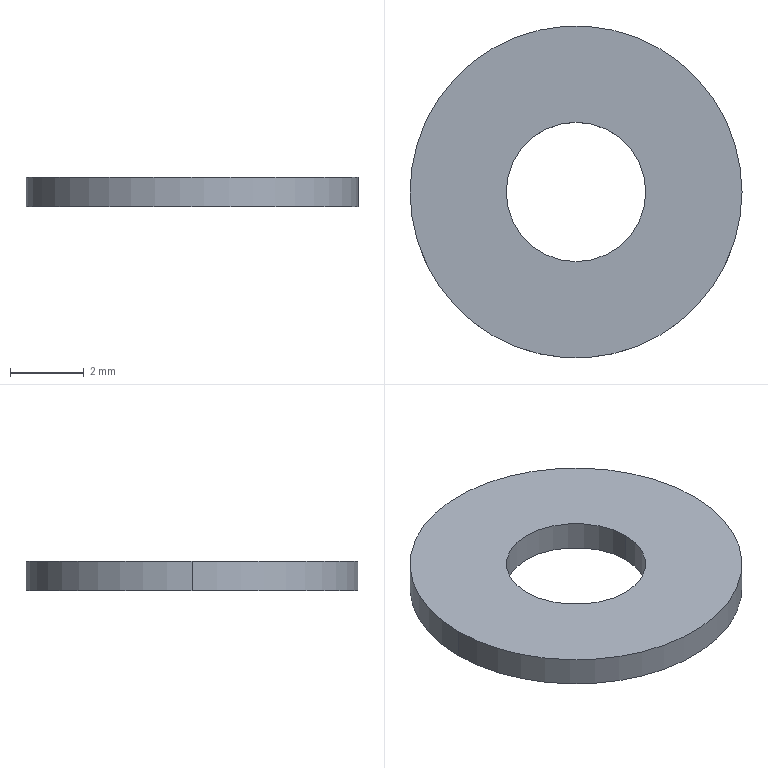Part | NX | features BREP 1 | 1 solid | 6 faces | box 9 x 9 x 0.8 mm | volume 41.916 mm3 | cylinder 4 | plane 2 | commonest cylinder face diameters 3.78 x2 9 x2
STEP:
#1=CARTESIAN_POINT('',(-264.811,-198.403,2105.2));
#2=VERTEX_POINT('',#1);
#3=CARTESIAN_POINT('',(-255.811,-198.403,2105.2));
#4=VERTEX_POINT('',#3);
#5=CARTESIAN_POINT('',(-260.311,-198.403,2105.2));
#6=DIRECTION('',(0.,0.,-1.));
#7=DIRECTION('',(1.,0.,0.));
#8=AXIS2_PLACEMENT_3D('',#5,#6,#7);
#9=CIRCLE('',#8,4.5);
#10=EDGE_CURVE('',#2,#4,#9,.T.);
#11=ORIENTED_EDGE('',*,*,#10,.F.);
#12=CARTESIAN_POINT('',(-264.811,-198.403,2106.));
#13=VERTEX_POINT('',#12);
#14=CARTESIAN_POINT('',(-264.811,-198.403,2106.));
#15=DIRECTION('',(0.,0.,1.));
#16=VECTOR('',#15,1000.);
#17=LINE('',#14,#16);
#18=EDGE_CURVE('',#2,#13,#17,.T.);
#19=ORIENTED_EDGE('',*,*,#18,.T.);
#20=CARTESIAN_POINT('',(-255.811,-198.403,2106.));
#21=VERTEX_POINT('',#20);
#22=CARTESIAN_POINT('',(-260.311,-198.403,2106.));
#23=DIRECTION('',(0.,0.,-1.));
#24=DIRECTION('',(1.,0.,0.));
#25=AXIS2_PLACEMENT_3D('',#22,#23,#24);
#26=CIRCLE('',#25,4.5);
#27=EDGE_CURVE('',#13,#21,#26,.T.);
#28=ORIENTED_EDGE('',*,*,#27,.T.);
#29=CARTESIAN_POINT('',(-255.811,-198.403,2106.));
#30=DIRECTION('',(0.,0.,1.));
#31=VECTOR('',#30,1000.);
#32=LINE('',#29,#31);
#33=EDGE_CURVE('',#4,#21,#32,.T.);
#34=ORIENTED_EDGE('',*,*,#33,.F.);
#35=EDGE_LOOP('',(#11,#19,#28,#34));
#36=FACE_BOUND('',#35,.T.);
#37=CARTESIAN_POINT('',(-260.311,-198.403,2106.));
#38=DIRECTION('',(0.,0.,1.));
#39=DIRECTION('',(-1.,0.,0.));
#40=AXIS2_PLACEMENT_3D('',#37,#38,#39);
#41=CYLINDRICAL_SURFACE('',#40,4.5);
#42=ADVANCED_FACE('',(#36),#41,.T.);
#43=CARTESIAN_POINT('',(-262.201,-198.403,2105.2));
#44=VERTEX_POINT('',#43);
#45=CARTESIAN_POINT('',(-258.421,-198.403,2105.2));
#46=VERTEX_POINT('',#45);
#47=CARTESIAN_POINT('',(-260.311,-198.403,2105.2));
#48=DIRECTION('',(0.,0.,1.));
#49=DIRECTION('',(1.,0.,0.));
#50=AXIS2_PLACEMENT_3D('',#47,#48,#49);
#51=CIRCLE('',#50,1.89);
#52=EDGE_CURVE('',#44,#46,#51,.T.);
#53=ORIENTED_EDGE('',*,*,#52,.F.);
#54=CARTESIAN_POINT('',(-262.201,-198.403,2106.));
#55=VERTEX_POINT('',#54);
#56=CARTESIAN_POINT('',(-262.201,-198.403,2106.));
#57=DIRECTION('',(0.,0.,1.));
#58=VECTOR('',#57,1000.);
#59=LINE('',#56,#58);
#60=EDGE_CURVE('',#44,#55,#59,.T.);
#61=ORIENTED_EDGE('',*,*,#60,.T.);
#62=CARTESIAN_POINT('',(-258.421,-198.403,2106.));
#63=VERTEX_POINT('',#62);
#64=CARTESIAN_POINT('',(-260.311,-198.403,2106.));
#65=DIRECTION('',(0.,0.,-1.));
#66=DIRECTION('',(1.,0.,0.));
#67=AXIS2_PLACEMENT_3D('',#64,#65,#66);
#68=CIRCLE('',#67,1.89);
#69=EDGE_CURVE('',#63,#55,#68,.T.);
#70=ORIENTED_EDGE('',*,*,#69,.F.);
#71=CARTESIAN_POINT('',(-258.421,-198.403,2106.));
#72=DIRECTION('',(0.,0.,1.));
#73=VECTOR('',#72,1000.);
#74=LINE('',#71,#73);
#75=EDGE_CURVE('',#46,#63,#74,.T.);
#76=ORIENTED_EDGE('',*,*,#75,.F.);
#77=EDGE_LOOP('',(#53,#61,#70,#76));
#78=FACE_BOUND('',#77,.T.);
#79=CARTESIAN_POINT('',(-260.311,-198.403,2106.));
#80=DIRECTION('',(0.,0.,1.));
#81=DIRECTION('',(-1.,0.,0.));
#82=AXIS2_PLACEMENT_3D('',#79,#80,#81);
#83=CYLINDRICAL_SURFACE('',#82,1.89);
#84=ADVANCED_FACE('',(#78),#83,.F.);
#85=CARTESIAN_POINT('',(-260.311,-198.403,2105.2));
#86=DIRECTION('',(0.,0.,-1.));
#87=DIRECTION('',(1.,0.,0.));
#88=AXIS2_PLACEMENT_3D('',#85,#86,#87);
#89=CIRCLE('',#88,4.5);
#90=EDGE_CURVE('',#4,#2,#89,.T.);
#91=ORIENTED_EDGE('',*,*,#90,.T.);
#92=ORIENTED_EDGE('',*,*,#10,.T.);
#93=EDGE_LOOP('',(#91,#92));
#94=FACE_BOUND('',#93,.T.);
#95=CARTESIAN_POINT('',(-260.311,-198.403,2105.2));
#96=DIRECTION('',(0.,0.,1.));
#97=DIRECTION('',(1.,0.,0.));
#98=AXIS2_PLACEMENT_3D('',#95,#96,#97);
#99=CIRCLE('',#98,1.89);
#100=EDGE_CURVE('',#46,#44,#99,.T.);
#101=ORIENTED_EDGE('',*,*,#100,.T.);
#102=ORIENTED_EDGE('',*,*,#52,.T.);
#103=EDGE_LOOP('',(#101,#102));
#104=FACE_BOUND('',#103,.T.);
#105=CARTESIAN_POINT('',(-260.302,-196.513,2105.2));
#106=DIRECTION('',(0.,0.,-1.));
#107=DIRECTION('',(1.,0.,0.));
#108=AXIS2_PLACEMENT_3D('',#105,#106,#107);
#109=PLANE('',#108);
#110=ADVANCED_FACE('',(#94,#104),#109,.T.);
#111=ORIENTED_EDGE('',*,*,#18,.F.);
#112=ORIENTED_EDGE('',*,*,#90,.F.);
#113=ORIENTED_EDGE('',*,*,#33,.T.);
#114=CARTESIAN_POINT('',(-260.311,-198.403,2106.));
#115=DIRECTION('',(0.,0.,-1.));
#116=DIRECTION('',(1.,0.,0.));
#117=AXIS2_PLACEMENT_3D('',#114,#115,#116);
#118=CIRCLE('',#117,4.5);
#119=EDGE_CURVE('',#21,#13,#118,.T.);
#120=ORIENTED_EDGE('',*,*,#119,.T.);
#121=EDGE_LOOP('',(#111,#112,#113,#120));
#122=FACE_BOUND('',#121,.T.);
#123=CARTESIAN_POINT('',(-260.311,-198.403,2106.));
#124=DIRECTION('',(0.,0.,1.));
#125=DIRECTION('',(-1.,0.,0.));
#126=AXIS2_PLACEMENT_3D('',#123,#124,#125);
#127=CYLINDRICAL_SURFACE('',#126,4.5);
#128=ADVANCED_FACE('',(#122),#127,.T.);
#129=ORIENTED_EDGE('',*,*,#60,.F.);
#130=ORIENTED_EDGE('',*,*,#100,.F.);
#131=ORIENTED_EDGE('',*,*,#75,.T.);
#132=CARTESIAN_POINT('',(-260.311,-198.403,2106.));
#133=DIRECTION('',(0.,0.,-1.));
#134=DIRECTION('',(1.,0.,0.));
#135=AXIS2_PLACEMENT_3D('',#132,#133,#134);
#136=CIRCLE('',#135,1.89);
#137=EDGE_CURVE('',#55,#63,#136,.T.);
#138=ORIENTED_EDGE('',*,*,#137,.F.);
#139=EDGE_LOOP('',(#129,#130,#131,#138));
#140=FACE_BOUND('',#139,.T.);
#141=CARTESIAN_POINT('',(-260.311,-198.403,2106.));
#142=DIRECTION('',(0.,0.,1.));
#143=DIRECTION('',(-1.,0.,0.));
#144=AXIS2_PLACEMENT_3D('',#141,#142,#143);
#145=CYLINDRICAL_SURFACE('',#144,1.89);
#146=ADVANCED_FACE('',(#140),#145,.F.);
#147=ORIENTED_EDGE('',*,*,#119,.F.);
#148=ORIENTED_EDGE('',*,*,#27,.F.);
#149=EDGE_LOOP('',(#147,#148));
#150=FACE_BOUND('',#149,.T.);
#151=ORIENTED_EDGE('',*,*,#69,.T.);
#152=ORIENTED_EDGE('',*,*,#137,.T.);
#153=EDGE_LOOP('',(#151,#152));
#154=FACE_BOUND('',#153,.T.);
#155=CARTESIAN_POINT('',(-260.302,-196.513,2106.));
#156=DIRECTION('',(0.,0.,1.));
#157=DIRECTION('',(-1.,0.,0.));
#158=AXIS2_PLACEMENT_3D('',#155,#156,#157);
#159=PLANE('',#158);
#160=ADVANCED_FACE('',(#150,#154),#159,.T.);
#161=CLOSED_SHELL('',(#42,#84,#110,#128,#146,#160));
#162=MANIFOLD_SOLID_BREP('',#161);
#163=(LENGTH_UNIT()NAMED_UNIT(*)SI_UNIT(.MILLI.,.METRE.));
#164=UNCERTAINTY_MEASURE_WITH_UNIT(LENGTH_MEASURE(0.00001),#163,'','');
#165=(NAMED_UNIT(*)PLANE_ANGLE_UNIT()SI_UNIT($,.RADIAN.));
#166=(NAMED_UNIT(*)SI_UNIT($,.STERADIAN.)SOLID_ANGLE_UNIT());
#167=(GEOMETRIC_REPRESENTATION_CONTEXT(3)GLOBAL_UNCERTAINTY_ASSIGNED_CONTEXT((#164))GLOBAL_UNIT_ASSIGNED_CONTEXT((#163,#165,#166))REPRESENTATION_CONTEXT('',''));
#168=ADVANCED_BREP_SHAPE_REPRESENTATION('',(#162),#167);